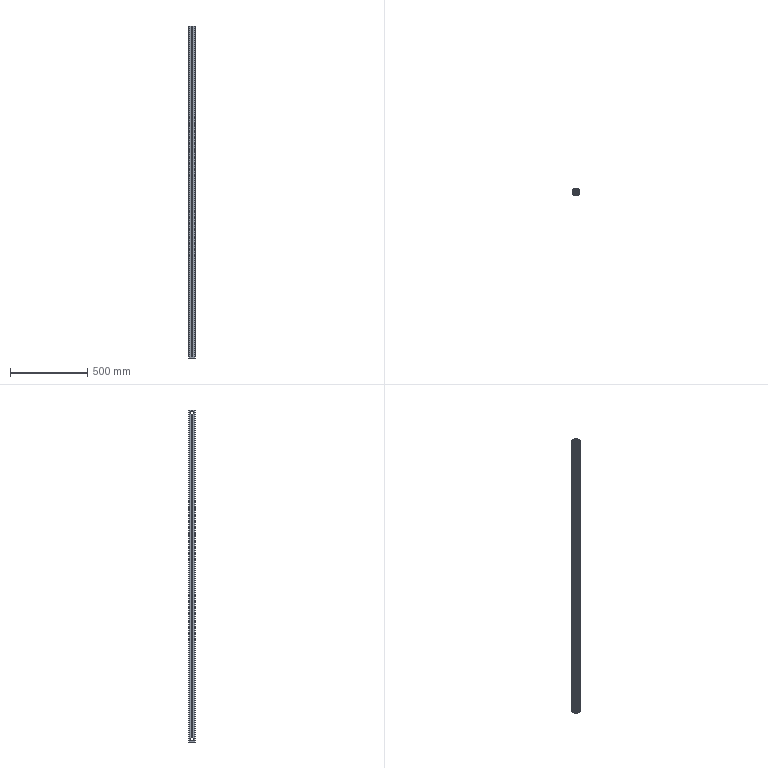Part | SolidWorks | features Extrusion 1, HoleWzd 1 | 1 solid | 273 faces | box 40 x 40 x 2144 mm | volume 1280370 mm3 | plane 213 | cylinder 60 | commonest cylinder face diameters 2 x16 6.8 x15 19 x12 1 x8 5 x4 9 x4